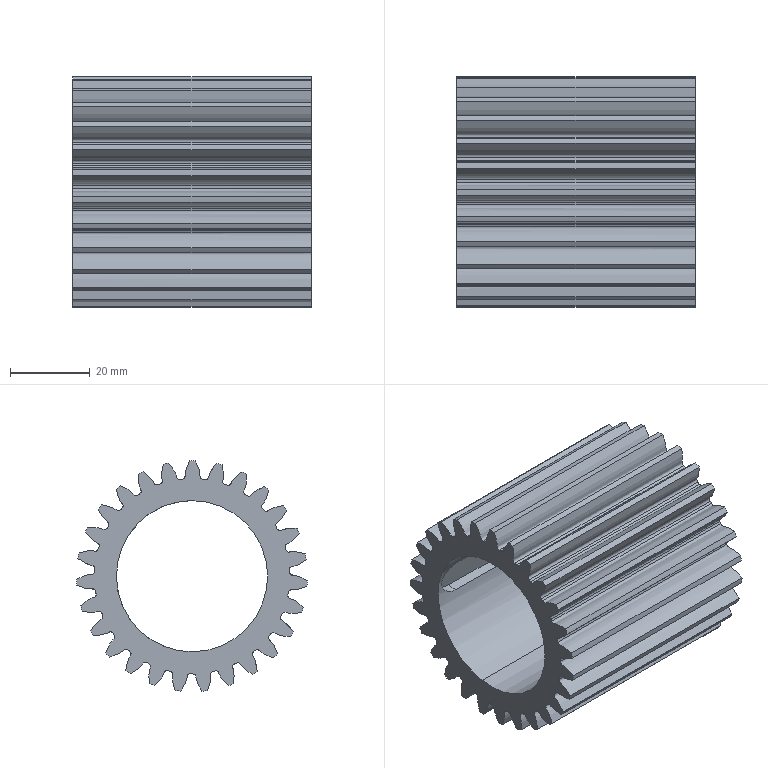Part | STEP file | Cut-Extrude 6 | 1 solid | 117 faces | box 60 x 57.967 x 57.893 mm | volume 66248 mm3 | cylinder 58 | spline 54 | plane 5 | commonest cylinder face diameters 49 x27 58 x27 10 x2 38 x2